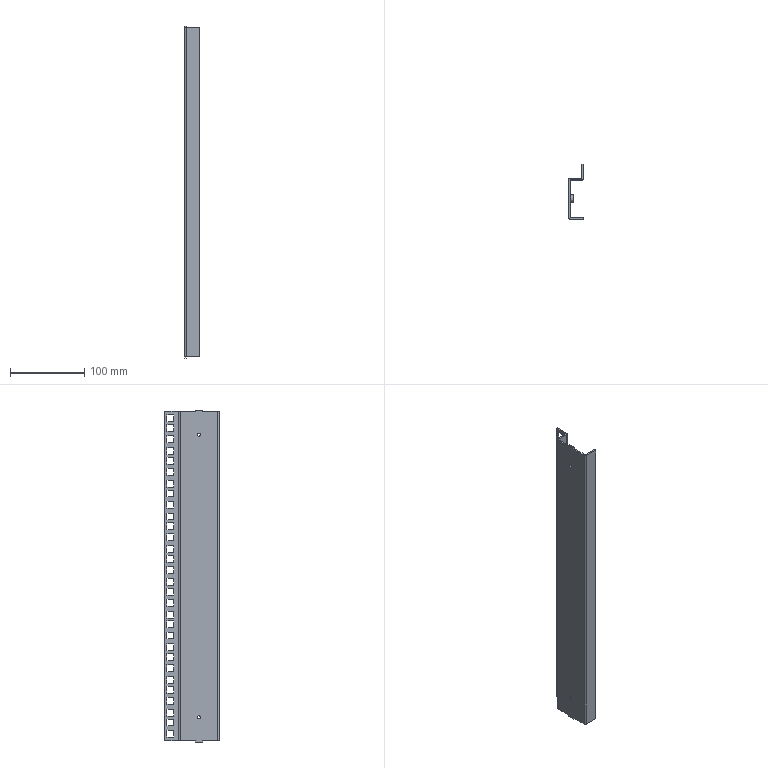Part | STEP file | FHD-021-001-O rack welded part O | 1 solid | 152 faces | box 20 x 73.5 x 446.5 mm | volume 91052 mm3 | plane 142 | cylinder 10 | commonest cylinder face diameters 0.4 x3 4.4 x3 4.2 x2 10.2 x2